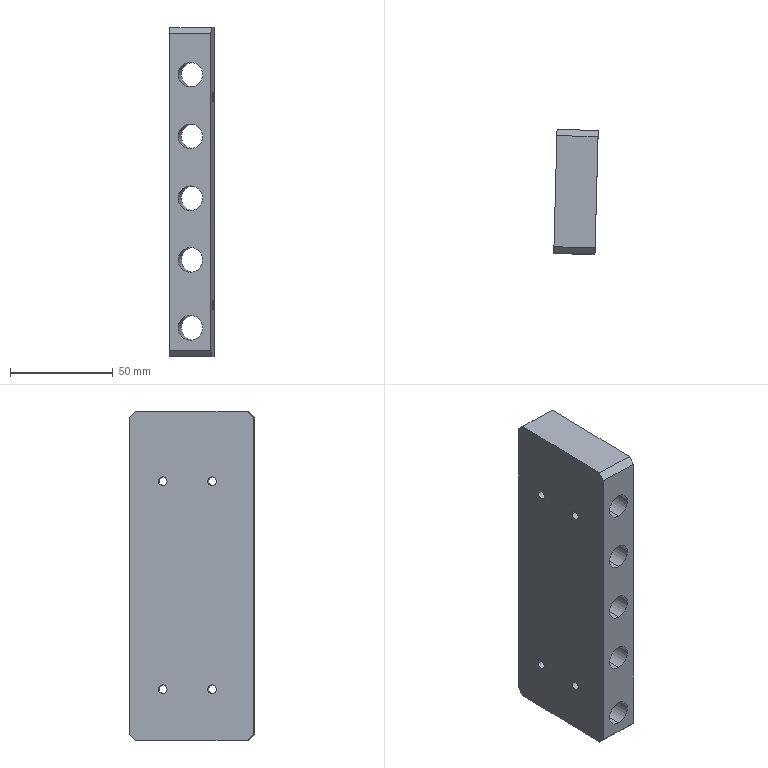Part | STEP file | 555 | 1 solid | 28 faces | box 21.564 x 60.503 x 160 mm | volume 156549 mm3 | cylinder 18 | plane 10 | commonest cylinder face diameters 12 x10 4.3 x8